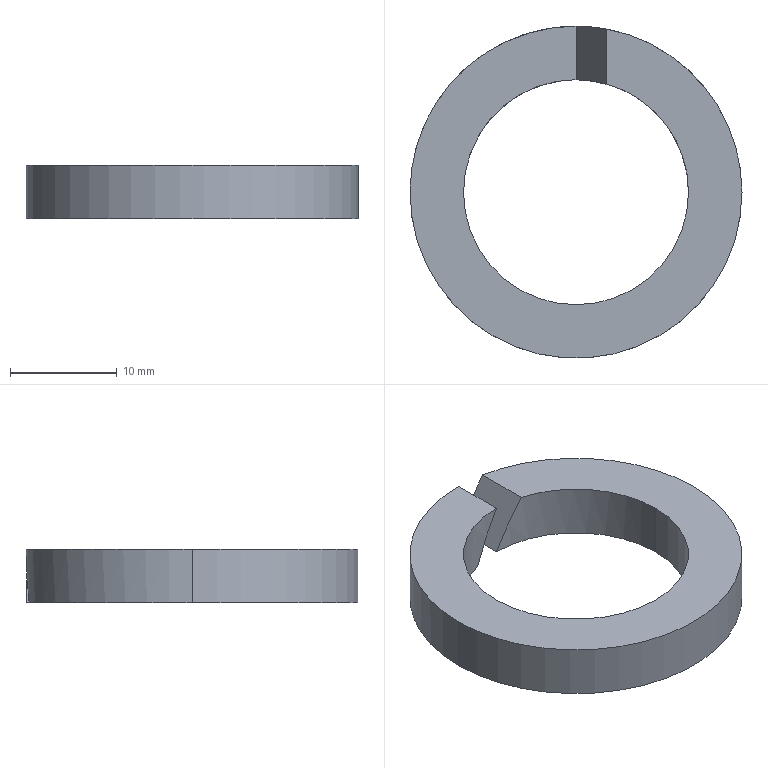Part | STEP file | Spring lock washers--Normal1 type GB_GB_FASTENER_WASHER_SW 20 | 1 solid | 10 faces | box 31.04 x 31.04 x 5 mm | volume 1973 mm3 | cylinder 6 | plane 4 | commonest cylinder face diameters 21.04 x3 31.04 x3
STEP:
#1=CARTESIAN_POINT('',(-10.52,0.,-5.));
#2=VERTEX_POINT('',#1);
#3=CARTESIAN_POINT('',(10.52,0.,-5.));
#4=VERTEX_POINT('',#3);
#5=CARTESIAN_POINT('',(0.,0.,-5.));
#6=DIRECTION('',(0.,0.,1.));
#7=DIRECTION('',(1.,0.,0.));
#8=AXIS2_PLACEMENT_3D('',#5,#6,#7);
#9=CIRCLE('',#8,10.52);
#10=EDGE_CURVE('',#2,#4,#9,.T.);
#11=ORIENTED_EDGE('',*,*,#10,.F.);
#12=CARTESIAN_POINT('',(-10.52,0.,0.));
#13=VERTEX_POINT('',#12);
#14=CARTESIAN_POINT('',(-10.52,0.,-5.));
#15=DIRECTION('',(0.,0.,1.));
#16=VECTOR('',#15,1000.);
#17=LINE('',#14,#16);
#18=EDGE_CURVE('',#2,#13,#17,.T.);
#19=ORIENTED_EDGE('',*,*,#18,.T.);
#20=CARTESIAN_POINT('',(10.52,0.,0.));
#21=VERTEX_POINT('',#20);
#22=CARTESIAN_POINT('',(0.,0.,0.));
#23=DIRECTION('',(0.,0.,-1.));
#24=DIRECTION('',(1.,0.,0.));
#25=AXIS2_PLACEMENT_3D('',#22,#23,#24);
#26=CIRCLE('',#25,10.52);
#27=EDGE_CURVE('',#21,#13,#26,.T.);
#28=ORIENTED_EDGE('',*,*,#27,.F.);
#29=CARTESIAN_POINT('',(10.52,0.,-5.));
#30=DIRECTION('',(0.,0.,1.));
#31=VECTOR('',#30,1000.);
#32=LINE('',#29,#31);
#33=EDGE_CURVE('',#4,#21,#32,.T.);
#34=ORIENTED_EDGE('',*,*,#33,.F.);
#35=EDGE_LOOP('',(#11,#19,#28,#34));
#36=FACE_OUTER_BOUND('',#35,.T.);
#37=CARTESIAN_POINT('',(0.,0.,-5.));
#38=DIRECTION('',(0.,0.,1.));
#39=DIRECTION('',(1.,0.,0.));
#40=AXIS2_PLACEMENT_3D('',#37,#38,#39);
#41=CYLINDRICAL_SURFACE('',#40,10.52);
#42=ADVANCED_FACE('',(#36),#41,.F.);
#43=CARTESIAN_POINT('',(0.,10.52,-5.));
#44=VERTEX_POINT('',#43);
#45=CARTESIAN_POINT('',(0.,0.,-5.));
#46=DIRECTION('',(0.,0.,1.));
#47=DIRECTION('',(1.,0.,0.));
#48=AXIS2_PLACEMENT_3D('',#45,#46,#47);
#49=CIRCLE('',#48,10.52);
#50=EDGE_CURVE('',#4,#44,#49,.T.);
#51=ORIENTED_EDGE('',*,*,#50,.F.);
#52=ORIENTED_EDGE('',*,*,#33,.T.);
#53=CARTESIAN_POINT('',(2.887,10.116,0.));
#54=VERTEX_POINT('',#53);
#55=CARTESIAN_POINT('',(0.,0.,0.));
#56=DIRECTION('',(0.,0.,-1.));
#57=DIRECTION('',(1.,0.,0.));
#58=AXIS2_PLACEMENT_3D('',#55,#56,#57);
#59=CIRCLE('',#58,10.52);
#60=EDGE_CURVE('',#54,#21,#59,.T.);
#61=ORIENTED_EDGE('',*,*,#60,.F.);
#62=CARTESIAN_POINT('',(0.,10.52,-5.));
#63=CARTESIAN_POINT('',(0.9779,10.52,-3.306));
#64=CARTESIAN_POINT('',(1.946,10.385,-1.629));
#65=CARTESIAN_POINT('',(2.887,10.116,0.));
#66=(BOUNDED_CURVE()B_SPLINE_CURVE(3,(#62,#63,#64,#65),.UNSPECIFIED.,.F.,.F.)B_SPLINE_CURVE_WITH_KNOTS((4,4),(4.712,4.99),.UNSPECIFIED.)CURVE()GEOMETRIC_REPRESENTATION_ITEM()RATIONAL_B_SPLINE_CURVE((1.,0.9936,0.9936,1.))REPRESENTATION_ITEM(''));
#67=EDGE_CURVE('',#44,#54,#66,.T.);
#68=ORIENTED_EDGE('',*,*,#67,.F.);
#69=EDGE_LOOP('',(#51,#52,#61,#68));
#70=FACE_OUTER_BOUND('',#69,.T.);
#71=CARTESIAN_POINT('',(0.,0.,-5.));
#72=DIRECTION('',(0.,0.,1.));
#73=DIRECTION('',(1.,0.,0.));
#74=AXIS2_PLACEMENT_3D('',#71,#72,#73);
#75=CYLINDRICAL_SURFACE('',#74,10.52);
#76=ADVANCED_FACE('',(#70),#75,.F.);
#77=CARTESIAN_POINT('',(-2.887,15.249,-5.));
#78=VERTEX_POINT('',#77);
#79=CARTESIAN_POINT('',(-15.52,0.,-5.));
#80=VERTEX_POINT('',#79);
#81=CARTESIAN_POINT('',(0.,0.,-5.));
#82=DIRECTION('',(0.,0.,1.));
#83=DIRECTION('',(1.,0.,0.));
#84=AXIS2_PLACEMENT_3D('',#81,#82,#83);
#85=CIRCLE('',#84,15.52);
#86=EDGE_CURVE('',#78,#80,#85,.T.);
#87=ORIENTED_EDGE('',*,*,#86,.T.);
#88=CARTESIAN_POINT('',(-15.52,0.,0.));
#89=VERTEX_POINT('',#88);
#90=CARTESIAN_POINT('',(-15.52,0.,-5.));
#91=DIRECTION('',(0.,0.,1.));
#92=VECTOR('',#91,1000.);
#93=LINE('',#90,#92);
#94=EDGE_CURVE('',#80,#89,#93,.T.);
#95=ORIENTED_EDGE('',*,*,#94,.T.);
#96=CARTESIAN_POINT('',(0.,15.52,0.));
#97=VERTEX_POINT('',#96);
#98=CARTESIAN_POINT('',(0.,0.,0.));
#99=DIRECTION('',(0.,0.,1.));
#100=DIRECTION('',(1.,0.,0.));
#101=AXIS2_PLACEMENT_3D('',#98,#99,#100);
#102=CIRCLE('',#101,15.52);
#103=EDGE_CURVE('',#97,#89,#102,.T.);
#104=ORIENTED_EDGE('',*,*,#103,.F.);
#105=CARTESIAN_POINT('',(0.,15.52,0.));
#106=CARTESIAN_POINT('',(-0.9693,15.52,-1.679));
#107=CARTESIAN_POINT('',(-1.934,15.429,-3.35));
#108=CARTESIAN_POINT('',(-2.887,15.249,-5.));
#109=(BOUNDED_CURVE()B_SPLINE_CURVE(3,(#105,#106,#107,#108),.UNSPECIFIED.,.F.,.F.)B_SPLINE_CURVE_WITH_KNOTS((4,4),(1.571,1.758),.UNSPECIFIED.)CURVE()GEOMETRIC_REPRESENTATION_ITEM()RATIONAL_B_SPLINE_CURVE((1.,0.9971,0.9971,1.))REPRESENTATION_ITEM(''));
#110=EDGE_CURVE('',#97,#78,#109,.T.);
#111=ORIENTED_EDGE('',*,*,#110,.T.);
#112=EDGE_LOOP('',(#87,#95,#104,#111));
#113=FACE_OUTER_BOUND('',#112,.T.);
#114=CARTESIAN_POINT('',(0.,0.,-5.));
#115=DIRECTION('',(0.,0.,1.));
#116=DIRECTION('',(1.,0.,0.));
#117=AXIS2_PLACEMENT_3D('',#114,#115,#116);
#118=CYLINDRICAL_SURFACE('',#117,15.52);
#119=ADVANCED_FACE('',(#113),#118,.T.);
#120=ORIENTED_EDGE('',*,*,#94,.F.);
#121=CARTESIAN_POINT('',(15.52,0.,-5.));
#122=VERTEX_POINT('',#121);
#123=CARTESIAN_POINT('',(0.,0.,-5.));
#124=DIRECTION('',(0.,0.,1.));
#125=DIRECTION('',(1.,0.,0.));
#126=AXIS2_PLACEMENT_3D('',#123,#124,#125);
#127=CIRCLE('',#126,15.52);
#128=EDGE_CURVE('',#80,#122,#127,.T.);
#129=ORIENTED_EDGE('',*,*,#128,.T.);
#130=CARTESIAN_POINT('',(15.52,0.,0.));
#131=VERTEX_POINT('',#130);
#132=CARTESIAN_POINT('',(15.52,0.,-5.));
#133=DIRECTION('',(0.,0.,1.));
#134=VECTOR('',#133,1000.);
#135=LINE('',#132,#134);
#136=EDGE_CURVE('',#122,#131,#135,.T.);
#137=ORIENTED_EDGE('',*,*,#136,.T.);
#138=CARTESIAN_POINT('',(0.,0.,0.));
#139=DIRECTION('',(0.,0.,1.));
#140=DIRECTION('',(1.,0.,0.));
#141=AXIS2_PLACEMENT_3D('',#138,#139,#140);
#142=CIRCLE('',#141,15.52);
#143=EDGE_CURVE('',#89,#131,#142,.T.);
#144=ORIENTED_EDGE('',*,*,#143,.F.);
#145=EDGE_LOOP('',(#120,#129,#137,#144));
#146=FACE_OUTER_BOUND('',#145,.T.);
#147=CARTESIAN_POINT('',(0.,0.,-5.));
#148=DIRECTION('',(0.,0.,1.));
#149=DIRECTION('',(1.,0.,0.));
#150=AXIS2_PLACEMENT_3D('',#147,#148,#149);
#151=CYLINDRICAL_SURFACE('',#150,15.52);
#152=ADVANCED_FACE('',(#146),#151,.T.);
#153=CARTESIAN_POINT('',(2.887,15.249,0.));
#154=VERTEX_POINT('',#153);
#155=CARTESIAN_POINT('',(2.887,0.,0.));
#156=DIRECTION('',(0.,-1.,0.));
#157=VECTOR('',#156,1000.);
#158=LINE('',#155,#157);
#159=EDGE_CURVE('',#154,#54,#158,.T.);
#160=ORIENTED_EDGE('',*,*,#159,.T.);
#161=ORIENTED_EDGE('',*,*,#60,.T.);
#162=ORIENTED_EDGE('',*,*,#27,.T.);
#163=CARTESIAN_POINT('',(0.,10.52,0.));
#164=VERTEX_POINT('',#163);
#165=CARTESIAN_POINT('',(0.,0.,0.));
#166=DIRECTION('',(0.,0.,-1.));
#167=DIRECTION('',(1.,0.,0.));
#168=AXIS2_PLACEMENT_3D('',#165,#166,#167);
#169=CIRCLE('',#168,10.52);
#170=EDGE_CURVE('',#13,#164,#169,.T.);
#171=ORIENTED_EDGE('',*,*,#170,.T.);
#172=CARTESIAN_POINT('',(0.,0.,0.));
#173=DIRECTION('',(0.,1.,0.));
#174=VECTOR('',#173,1000.);
#175=LINE('',#172,#174);
#176=EDGE_CURVE('',#164,#97,#175,.T.);
#177=ORIENTED_EDGE('',*,*,#176,.T.);
#178=ORIENTED_EDGE('',*,*,#103,.T.);
#179=ORIENTED_EDGE('',*,*,#143,.T.);
#180=CARTESIAN_POINT('',(0.,0.,0.));
#181=DIRECTION('',(0.,0.,1.));
#182=DIRECTION('',(1.,0.,0.));
#183=AXIS2_PLACEMENT_3D('',#180,#181,#182);
#184=CIRCLE('',#183,15.52);
#185=EDGE_CURVE('',#131,#154,#184,.T.);
#186=ORIENTED_EDGE('',*,*,#185,.T.);
#187=EDGE_LOOP('',(#160,#161,#162,#171,#177,#178,#179,#186));
#188=FACE_OUTER_BOUND('',#187,.T.);
#189=CARTESIAN_POINT('',(0.,0.,0.));
#190=DIRECTION('',(0.,0.,1.));
#191=DIRECTION('',(1.,0.,0.));
#192=AXIS2_PLACEMENT_3D('',#189,#190,#191);
#193=PLANE('',#192);
#194=ADVANCED_FACE('',(#188),#193,.T.);
#195=ORIENTED_EDGE('',*,*,#18,.F.);
#196=CARTESIAN_POINT('',(-2.887,10.116,-5.));
#197=VERTEX_POINT('',#196);
#198=CARTESIAN_POINT('',(0.,0.,-5.));
#199=DIRECTION('',(0.,0.,1.));
#200=DIRECTION('',(1.,0.,0.));
#201=AXIS2_PLACEMENT_3D('',#198,#199,#200);
#202=CIRCLE('',#201,10.52);
#203=EDGE_CURVE('',#197,#2,#202,.T.);
#204=ORIENTED_EDGE('',*,*,#203,.F.);
#205=CARTESIAN_POINT('',(0.,10.52,0.));
#206=CARTESIAN_POINT('',(-0.9779,10.52,-1.694));
#207=CARTESIAN_POINT('',(-1.946,10.385,-3.371));
#208=CARTESIAN_POINT('',(-2.887,10.116,-5.));
#209=(BOUNDED_CURVE()B_SPLINE_CURVE(3,(#205,#206,#207,#208),.UNSPECIFIED.,.F.,.F.)B_SPLINE_CURVE_WITH_KNOTS((4,4),(1.571,1.849),.UNSPECIFIED.)CURVE()GEOMETRIC_REPRESENTATION_ITEM()RATIONAL_B_SPLINE_CURVE((1.,0.9936,0.9936,1.))REPRESENTATION_ITEM(''));
#210=EDGE_CURVE('',#164,#197,#209,.T.);
#211=ORIENTED_EDGE('',*,*,#210,.F.);
#212=ORIENTED_EDGE('',*,*,#170,.F.);
#213=EDGE_LOOP('',(#195,#204,#211,#212));
#214=FACE_OUTER_BOUND('',#213,.T.);
#215=CARTESIAN_POINT('',(0.,0.,-5.));
#216=DIRECTION('',(0.,0.,1.));
#217=DIRECTION('',(1.,0.,0.));
#218=AXIS2_PLACEMENT_3D('',#215,#216,#217);
#219=CYLINDRICAL_SURFACE('',#218,10.52);
#220=ADVANCED_FACE('',(#214),#219,.F.);
#221=ORIENTED_EDGE('',*,*,#159,.F.);
#222=CARTESIAN_POINT('',(0.,15.52,-5.));
#223=VERTEX_POINT('',#222);
#224=CARTESIAN_POINT('',(2.887,15.249,0.));
#225=CARTESIAN_POINT('',(1.934,15.429,-1.65));
#226=CARTESIAN_POINT('',(0.9693,15.52,-3.321));
#227=CARTESIAN_POINT('',(0.,15.52,-5.));
#228=(BOUNDED_CURVE()B_SPLINE_CURVE(3,(#224,#225,#226,#227),.UNSPECIFIED.,.F.,.F.)B_SPLINE_CURVE_WITH_KNOTS((4,4),(1.384,1.571),.UNSPECIFIED.)CURVE()GEOMETRIC_REPRESENTATION_ITEM()RATIONAL_B_SPLINE_CURVE((1.,0.9971,0.9971,1.))REPRESENTATION_ITEM(''));
#229=EDGE_CURVE('',#154,#223,#228,.T.);
#230=ORIENTED_EDGE('',*,*,#229,.T.);
#231=CARTESIAN_POINT('',(0.,15.52,-5.));
#232=DIRECTION('',(0.,-1.,0.));
#233=VECTOR('',#232,1000.);
#234=LINE('',#231,#233);
#235=EDGE_CURVE('',#223,#44,#234,.T.);
#236=ORIENTED_EDGE('',*,*,#235,.T.);
#237=ORIENTED_EDGE('',*,*,#67,.T.);
#238=EDGE_LOOP('',(#221,#230,#236,#237));
#239=FACE_OUTER_BOUND('',#238,.T.);
#240=CARTESIAN_POINT('',(0.,15.52,-5.));
#241=DIRECTION('',(-0.866,0.,0.5));
#242=DIRECTION('',(0.5,0.,0.866));
#243=AXIS2_PLACEMENT_3D('',#240,#241,#242);
#244=PLANE('',#243);
#245=ADVANCED_FACE('',(#239),#244,.T.);
#246=ORIENTED_EDGE('',*,*,#136,.F.);
#247=CARTESIAN_POINT('',(0.,0.,-5.));
#248=DIRECTION('',(0.,0.,1.));
#249=DIRECTION('',(1.,0.,0.));
#250=AXIS2_PLACEMENT_3D('',#247,#248,#249);
#251=CIRCLE('',#250,15.52);
#252=EDGE_CURVE('',#122,#223,#251,.T.);
#253=ORIENTED_EDGE('',*,*,#252,.T.);
#254=ORIENTED_EDGE('',*,*,#229,.F.);
#255=ORIENTED_EDGE('',*,*,#185,.F.);
#256=EDGE_LOOP('',(#246,#253,#254,#255));
#257=FACE_OUTER_BOUND('',#256,.T.);
#258=CARTESIAN_POINT('',(0.,0.,-5.));
#259=DIRECTION('',(0.,0.,1.));
#260=DIRECTION('',(1.,0.,0.));
#261=AXIS2_PLACEMENT_3D('',#258,#259,#260);
#262=CYLINDRICAL_SURFACE('',#261,15.52);
#263=ADVANCED_FACE('',(#257),#262,.T.);
#264=CARTESIAN_POINT('',(-2.887,15.52,-5.));
#265=DIRECTION('',(0.,1.,0.));
#266=VECTOR('',#265,1000.);
#267=LINE('',#264,#266);
#268=EDGE_CURVE('',#197,#78,#267,.T.);
#269=ORIENTED_EDGE('',*,*,#268,.T.);
#270=ORIENTED_EDGE('',*,*,#110,.F.);
#271=ORIENTED_EDGE('',*,*,#176,.F.);
#272=ORIENTED_EDGE('',*,*,#210,.T.);
#273=EDGE_LOOP('',(#269,#270,#271,#272));
#274=FACE_OUTER_BOUND('',#273,.T.);
#275=CARTESIAN_POINT('',(0.,15.52,0.));
#276=DIRECTION('',(0.866,0.,-0.5));
#277=DIRECTION('',(-0.5,0.,-0.866));
#278=AXIS2_PLACEMENT_3D('',#275,#276,#277);
#279=PLANE('',#278);
#280=ADVANCED_FACE('',(#274),#279,.T.);
#281=ORIENTED_EDGE('',*,*,#268,.F.);
#282=ORIENTED_EDGE('',*,*,#203,.T.);
#283=ORIENTED_EDGE('',*,*,#10,.T.);
#284=ORIENTED_EDGE('',*,*,#50,.T.);
#285=ORIENTED_EDGE('',*,*,#235,.F.);
#286=ORIENTED_EDGE('',*,*,#252,.F.);
#287=ORIENTED_EDGE('',*,*,#128,.F.);
#288=ORIENTED_EDGE('',*,*,#86,.F.);
#289=EDGE_LOOP('',(#281,#282,#283,#284,#285,#286,#287,#288));
#290=FACE_OUTER_BOUND('',#289,.T.);
#291=CARTESIAN_POINT('',(0.,0.,-5.));
#292=DIRECTION('',(0.,0.,1.));
#293=DIRECTION('',(1.,0.,0.));
#294=AXIS2_PLACEMENT_3D('',#291,#292,#293);
#295=PLANE('',#294);
#296=ADVANCED_FACE('',(#290),#295,.F.);
#297=CLOSED_SHELL('',(#42,#76,#119,#152,#194,#220,#245,#263,#280,#296));
#298=MANIFOLD_SOLID_BREP('',#297);
#299=CARTESIAN_POINT('',(0.,0.,0.));
#300=DIRECTION('',(0.,0.,1.));
#301=DIRECTION('',(1.,0.,0.));
#302=AXIS2_PLACEMENT_3D('',#299,#300,#301);
#303=(LENGTH_UNIT()NAMED_UNIT(*)SI_UNIT(.MILLI.,.METRE.));
#304=UNCERTAINTY_MEASURE_WITH_UNIT(LENGTH_MEASURE(0.00001),#303,'','');
#305=(NAMED_UNIT(*)PLANE_ANGLE_UNIT()SI_UNIT($,.RADIAN.));
#306=(NAMED_UNIT(*)SI_UNIT($,.STERADIAN.)SOLID_ANGLE_UNIT());
#307=(GEOMETRIC_REPRESENTATION_CONTEXT(3)GLOBAL_UNCERTAINTY_ASSIGNED_CONTEXT((#304))GLOBAL_UNIT_ASSIGNED_CONTEXT((#303,#305,#306))REPRESENTATION_CONTEXT('',''));
#308=ADVANCED_BREP_SHAPE_REPRESENTATION('',(#298,#302),#307);